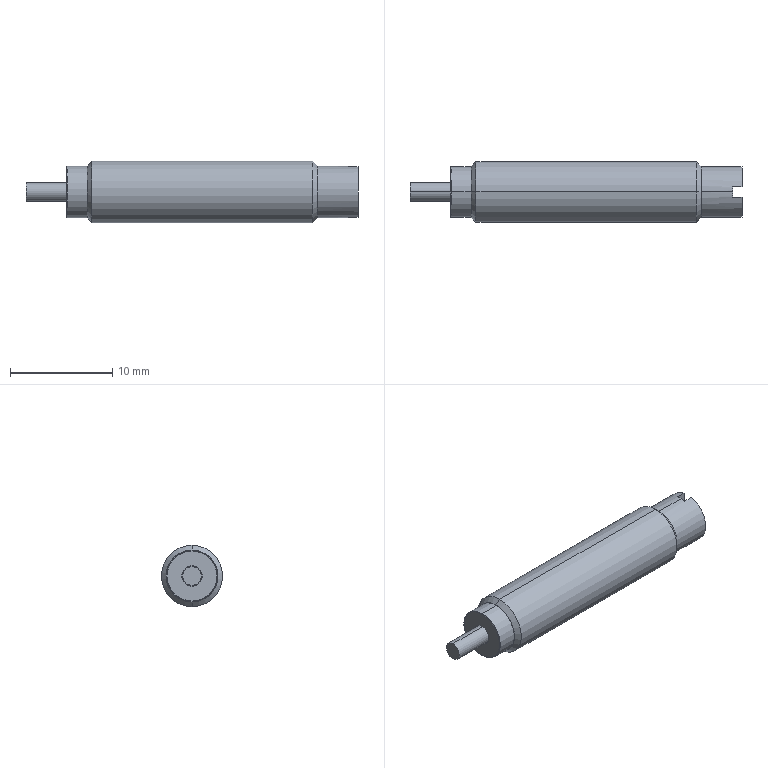Part | STEP file | 1_10 | 1 solid | 26 faces | box 32.5 x 6 x 6 mm | volume 755.606 mm3 | cylinder 10 | plane 10 | cone 4 | spline 2 | commonest cylinder face diameters 5 x4 1.8 x2 2 x2 6 x2